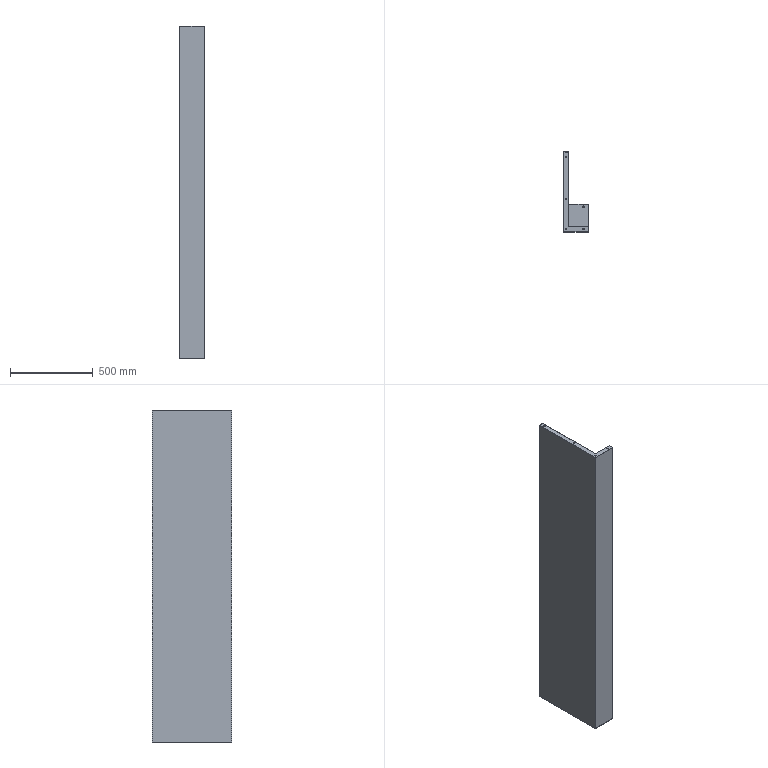Part | SolidWorks | features ICE 8, ExtruThin 1 | 1 solid | 45 faces | box 150 x 480 x 2005 mm | volume 2840339 mm3 | cylinder 30 | plane 15 | commonest cylinder face diameters 9 x30
STEP:
#1=CARTESIAN_POINT('',(148.,16.,1267.5));
#2=VERTEX_POINT('',#1);
#3=CARTESIAN_POINT('',(148.,16.,1258.5));
#4=VERTEX_POINT('',#3);
#5=CARTESIAN_POINT('',(148.,16.,1263.));
#6=DIRECTION('',(1.,0.,0.));
#7=DIRECTION('',(0.,0.,-1.));
#8=AXIS2_PLACEMENT_3D('',#5,#6,#7);
#9=CIRCLE('',#8,4.5);
#10=EDGE_CURVE('',#2,#4,#9,.T.);
#11=ORIENTED_EDGE('',*,*,#10,.F.);
#12=CARTESIAN_POINT('',(150.,16.,1267.5));
#13=VERTEX_POINT('',#12);
#14=CARTESIAN_POINT('',(134.,16.,1267.5));
#15=DIRECTION('',(1.,0.,0.));
#16=VECTOR('',#15,1000.);
#17=LINE('',#14,#16);
#18=EDGE_CURVE('',#2,#13,#17,.T.);
#19=ORIENTED_EDGE('',*,*,#18,.T.);
#20=CARTESIAN_POINT('',(150.,16.,1258.5));
#21=VERTEX_POINT('',#20);
#22=CARTESIAN_POINT('',(150.,16.,1263.));
#23=DIRECTION('',(1.,0.,0.));
#24=DIRECTION('',(0.,0.,-1.));
#25=AXIS2_PLACEMENT_3D('',#22,#23,#24);
#26=CIRCLE('',#25,4.5);
#27=EDGE_CURVE('',#13,#21,#26,.T.);
#28=ORIENTED_EDGE('',*,*,#27,.T.);
#29=CARTESIAN_POINT('',(134.,16.,1258.5));
#30=DIRECTION('',(1.,0.,0.));
#31=VECTOR('',#30,1000.);
#32=LINE('',#29,#31);
#33=EDGE_CURVE('',#4,#21,#32,.T.);
#34=ORIENTED_EDGE('',*,*,#33,.F.);
#35=EDGE_LOOP('',(#11,#19,#28,#34));
#36=FACE_OUTER_BOUND('',#35,.T.);
#37=CARTESIAN_POINT('',(134.,16.,1263.));
#38=DIRECTION('',(1.,0.,0.));
#39=DIRECTION('',(0.,0.,-1.));
#40=AXIS2_PLACEMENT_3D('',#37,#38,#39);
#41=CYLINDRICAL_SURFACE('',#40,4.5);
#42=ADVANCED_FACE('',(#36),#41,.F.);
#43=CARTESIAN_POINT('',(148.,16.,1335.5));
#44=VERTEX_POINT('',#43);
#45=CARTESIAN_POINT('',(148.,16.,1326.5));
#46=VERTEX_POINT('',#45);
#47=CARTESIAN_POINT('',(148.,16.,1331.));
#48=DIRECTION('',(1.,0.,0.));
#49=DIRECTION('',(0.,0.,-1.));
#50=AXIS2_PLACEMENT_3D('',#47,#48,#49);
#51=CIRCLE('',#50,4.5);
#52=EDGE_CURVE('',#44,#46,#51,.T.);
#53=ORIENTED_EDGE('',*,*,#52,.F.);
#54=CARTESIAN_POINT('',(150.,16.,1335.5));
#55=VERTEX_POINT('',#54);
#56=CARTESIAN_POINT('',(134.,16.,1335.5));
#57=DIRECTION('',(1.,0.,0.));
#58=VECTOR('',#57,1000.);
#59=LINE('',#56,#58);
#60=EDGE_CURVE('',#44,#55,#59,.T.);
#61=ORIENTED_EDGE('',*,*,#60,.T.);
#62=CARTESIAN_POINT('',(150.,16.,1326.5));
#63=VERTEX_POINT('',#62);
#64=CARTESIAN_POINT('',(150.,16.,1331.));
#65=DIRECTION('',(1.,0.,0.));
#66=DIRECTION('',(0.,0.,-1.));
#67=AXIS2_PLACEMENT_3D('',#64,#65,#66);
#68=CIRCLE('',#67,4.5);
#69=EDGE_CURVE('',#55,#63,#68,.T.);
#70=ORIENTED_EDGE('',*,*,#69,.T.);
#71=CARTESIAN_POINT('',(134.,16.,1326.5));
#72=DIRECTION('',(1.,0.,0.));
#73=VECTOR('',#72,1000.);
#74=LINE('',#71,#73);
#75=EDGE_CURVE('',#46,#63,#74,.T.);
#76=ORIENTED_EDGE('',*,*,#75,.F.);
#77=EDGE_LOOP('',(#53,#61,#70,#76));
#78=FACE_OUTER_BOUND('',#77,.T.);
#79=CARTESIAN_POINT('',(134.,16.,1331.));
#80=DIRECTION('',(1.,0.,0.));
#81=DIRECTION('',(0.,0.,-1.));
#82=AXIS2_PLACEMENT_3D('',#79,#80,#81);
#83=CYLINDRICAL_SURFACE('',#82,4.5);
#84=ADVANCED_FACE('',(#78),#83,.F.);
#85=CARTESIAN_POINT('',(148.,16.,34.5));
#86=VERTEX_POINT('',#85);
#87=CARTESIAN_POINT('',(148.,16.,25.5));
#88=VERTEX_POINT('',#87);
#89=CARTESIAN_POINT('',(148.,16.,30.));
#90=DIRECTION('',(1.,0.,0.));
#91=DIRECTION('',(0.,0.,-1.));
#92=AXIS2_PLACEMENT_3D('',#89,#90,#91);
#93=CIRCLE('',#92,4.5);
#94=EDGE_CURVE('',#86,#88,#93,.T.);
#95=ORIENTED_EDGE('',*,*,#94,.F.);
#96=CARTESIAN_POINT('',(150.,16.,34.5));
#97=VERTEX_POINT('',#96);
#98=CARTESIAN_POINT('',(134.,16.,34.5));
#99=DIRECTION('',(1.,0.,0.));
#100=VECTOR('',#99,1000.);
#101=LINE('',#98,#100);
#102=EDGE_CURVE('',#86,#97,#101,.T.);
#103=ORIENTED_EDGE('',*,*,#102,.T.);
#104=CARTESIAN_POINT('',(150.,16.,25.5));
#105=VERTEX_POINT('',#104);
#106=CARTESIAN_POINT('',(150.,16.,30.));
#107=DIRECTION('',(1.,0.,0.));
#108=DIRECTION('',(0.,0.,-1.));
#109=AXIS2_PLACEMENT_3D('',#106,#107,#108);
#110=CIRCLE('',#109,4.5);
#111=EDGE_CURVE('',#97,#105,#110,.T.);
#112=ORIENTED_EDGE('',*,*,#111,.T.);
#113=CARTESIAN_POINT('',(134.,16.,25.5));
#114=DIRECTION('',(1.,0.,0.));
#115=VECTOR('',#114,1000.);
#116=LINE('',#113,#115);
#117=EDGE_CURVE('',#88,#105,#116,.T.);
#118=ORIENTED_EDGE('',*,*,#117,.F.);
#119=EDGE_LOOP('',(#95,#103,#112,#118));
#120=FACE_OUTER_BOUND('',#119,.T.);
#121=CARTESIAN_POINT('',(134.,16.,30.));
#122=DIRECTION('',(1.,0.,0.));
#123=DIRECTION('',(0.,0.,-1.));
#124=AXIS2_PLACEMENT_3D('',#121,#122,#123);
#125=CYLINDRICAL_SURFACE('',#124,4.5);
#126=ADVANCED_FACE('',(#120),#125,.F.);
#127=CARTESIAN_POINT('',(148.,16.,179.5));
#128=VERTEX_POINT('',#127);
#129=CARTESIAN_POINT('',(148.,16.,170.5));
#130=VERTEX_POINT('',#129);
#131=CARTESIAN_POINT('',(148.,16.,175.));
#132=DIRECTION('',(1.,0.,0.));
#133=DIRECTION('',(0.,0.,-1.));
#134=AXIS2_PLACEMENT_3D('',#131,#132,#133);
#135=CIRCLE('',#134,4.5);
#136=EDGE_CURVE('',#128,#130,#135,.T.);
#137=ORIENTED_EDGE('',*,*,#136,.F.);
#138=CARTESIAN_POINT('',(150.,16.,179.5));
#139=VERTEX_POINT('',#138);
#140=CARTESIAN_POINT('',(134.,16.,179.5));
#141=DIRECTION('',(1.,0.,0.));
#142=VECTOR('',#141,1000.);
#143=LINE('',#140,#142);
#144=EDGE_CURVE('',#128,#139,#143,.T.);
#145=ORIENTED_EDGE('',*,*,#144,.T.);
#146=CARTESIAN_POINT('',(150.,16.,170.5));
#147=VERTEX_POINT('',#146);
#148=CARTESIAN_POINT('',(150.,16.,175.));
#149=DIRECTION('',(1.,0.,0.));
#150=DIRECTION('',(0.,0.,-1.));
#151=AXIS2_PLACEMENT_3D('',#148,#149,#150);
#152=CIRCLE('',#151,4.5);
#153=EDGE_CURVE('',#139,#147,#152,.T.);
#154=ORIENTED_EDGE('',*,*,#153,.T.);
#155=CARTESIAN_POINT('',(134.,16.,170.5));
#156=DIRECTION('',(1.,0.,0.));
#157=VECTOR('',#156,1000.);
#158=LINE('',#155,#157);
#159=EDGE_CURVE('',#130,#147,#158,.T.);
#160=ORIENTED_EDGE('',*,*,#159,.F.);
#161=EDGE_LOOP('',(#137,#145,#154,#160));
#162=FACE_OUTER_BOUND('',#161,.T.);
#163=CARTESIAN_POINT('',(134.,16.,175.));
#164=DIRECTION('',(1.,0.,0.));
#165=DIRECTION('',(0.,0.,-1.));
#166=AXIS2_PLACEMENT_3D('',#163,#164,#165);
#167=CYLINDRICAL_SURFACE('',#166,4.5);
#168=ADVANCED_FACE('',(#162),#167,.F.);
#169=CARTESIAN_POINT('',(115.5,16.,2003.));
#170=VERTEX_POINT('',#169);
#171=CARTESIAN_POINT('',(124.5,16.,2003.));
#172=VERTEX_POINT('',#171);
#173=CARTESIAN_POINT('',(120.,16.,2003.));
#174=DIRECTION('',(0.,0.,1.));
#175=DIRECTION('',(1.,0.,0.));
#176=AXIS2_PLACEMENT_3D('',#173,#174,#175);
#177=CIRCLE('',#176,4.5);
#178=EDGE_CURVE('',#170,#172,#177,.T.);
#179=ORIENTED_EDGE('',*,*,#178,.F.);
#180=CARTESIAN_POINT('',(115.5,16.,2005.));
#181=VERTEX_POINT('',#180);
#182=CARTESIAN_POINT('',(115.5,16.,1995.));
#183=DIRECTION('',(0.,0.,1.));
#184=VECTOR('',#183,1000.);
#185=LINE('',#182,#184);
#186=EDGE_CURVE('',#170,#181,#185,.T.);
#187=ORIENTED_EDGE('',*,*,#186,.T.);
#188=CARTESIAN_POINT('',(124.5,16.,2005.));
#189=VERTEX_POINT('',#188);
#190=CARTESIAN_POINT('',(120.,16.,2005.));
#191=DIRECTION('',(0.,0.,1.));
#192=DIRECTION('',(1.,0.,0.));
#193=AXIS2_PLACEMENT_3D('',#190,#191,#192);
#194=CIRCLE('',#193,4.5);
#195=EDGE_CURVE('',#181,#189,#194,.T.);
#196=ORIENTED_EDGE('',*,*,#195,.T.);
#197=CARTESIAN_POINT('',(124.5,16.,1995.));
#198=DIRECTION('',(0.,0.,1.));
#199=VECTOR('',#198,1000.);
#200=LINE('',#197,#199);
#201=EDGE_CURVE('',#172,#189,#200,.T.);
#202=ORIENTED_EDGE('',*,*,#201,.F.);
#203=EDGE_LOOP('',(#179,#187,#196,#202));
#204=FACE_OUTER_BOUND('',#203,.T.);
#205=CARTESIAN_POINT('',(120.,16.,1995.));
#206=DIRECTION('',(0.,0.,1.));
#207=DIRECTION('',(1.,0.,0.));
#208=AXIS2_PLACEMENT_3D('',#205,#206,#207);
#209=CYLINDRICAL_SURFACE('',#208,4.5);
#210=ADVANCED_FACE('',(#204),#209,.F.);
#211=CARTESIAN_POINT('',(11.5,16.,2003.));
#212=VERTEX_POINT('',#211);
#213=CARTESIAN_POINT('',(20.5,16.,2003.));
#214=VERTEX_POINT('',#213);
#215=CARTESIAN_POINT('',(16.,16.,2003.));
#216=DIRECTION('',(0.,0.,1.));
#217=DIRECTION('',(1.,0.,0.));
#218=AXIS2_PLACEMENT_3D('',#215,#216,#217);
#219=CIRCLE('',#218,4.5);
#220=EDGE_CURVE('',#212,#214,#219,.T.);
#221=ORIENTED_EDGE('',*,*,#220,.F.);
#222=CARTESIAN_POINT('',(11.5,16.,2005.));
#223=VERTEX_POINT('',#222);
#224=CARTESIAN_POINT('',(11.5,16.,1995.));
#225=DIRECTION('',(0.,0.,1.));
#226=VECTOR('',#225,1000.);
#227=LINE('',#224,#226);
#228=EDGE_CURVE('',#212,#223,#227,.T.);
#229=ORIENTED_EDGE('',*,*,#228,.T.);
#230=CARTESIAN_POINT('',(20.5,16.,2005.));
#231=VERTEX_POINT('',#230);
#232=CARTESIAN_POINT('',(16.,16.,2005.));
#233=DIRECTION('',(0.,0.,1.));
#234=DIRECTION('',(1.,0.,0.));
#235=AXIS2_PLACEMENT_3D('',#232,#233,#234);
#236=CIRCLE('',#235,4.5);
#237=EDGE_CURVE('',#223,#231,#236,.T.);
#238=ORIENTED_EDGE('',*,*,#237,.T.);
#239=CARTESIAN_POINT('',(20.5,16.,1995.));
#240=DIRECTION('',(0.,0.,1.));
#241=VECTOR('',#240,1000.);
#242=LINE('',#239,#241);
#243=EDGE_CURVE('',#214,#231,#242,.T.);
#244=ORIENTED_EDGE('',*,*,#243,.F.);
#245=EDGE_LOOP('',(#221,#229,#238,#244));
#246=FACE_OUTER_BOUND('',#245,.T.);
#247=CARTESIAN_POINT('',(16.,16.,1995.));
#248=DIRECTION('',(0.,0.,1.));
#249=DIRECTION('',(1.,0.,0.));
#250=AXIS2_PLACEMENT_3D('',#247,#248,#249);
#251=CYLINDRICAL_SURFACE('',#250,4.5);
#252=ADVANCED_FACE('',(#246),#251,.F.);
#253=CARTESIAN_POINT('',(11.5,197.,2003.));
#254=VERTEX_POINT('',#253);
#255=CARTESIAN_POINT('',(20.5,197.,2003.));
#256=VERTEX_POINT('',#255);
#257=CARTESIAN_POINT('',(16.,197.,2003.));
#258=DIRECTION('',(0.,0.,1.));
#259=DIRECTION('',(1.,0.,0.));
#260=AXIS2_PLACEMENT_3D('',#257,#258,#259);
#261=CIRCLE('',#260,4.5);
#262=EDGE_CURVE('',#254,#256,#261,.T.);
#263=ORIENTED_EDGE('',*,*,#262,.F.);
#264=CARTESIAN_POINT('',(11.5,197.,2005.));
#265=VERTEX_POINT('',#264);
#266=CARTESIAN_POINT('',(11.5,197.,1995.));
#267=DIRECTION('',(0.,0.,1.));
#268=VECTOR('',#267,1000.);
#269=LINE('',#266,#268);
#270=EDGE_CURVE('',#254,#265,#269,.T.);
#271=ORIENTED_EDGE('',*,*,#270,.T.);
#272=CARTESIAN_POINT('',(20.5,197.,2005.));
#273=VERTEX_POINT('',#272);
#274=CARTESIAN_POINT('',(16.,197.,2005.));
#275=DIRECTION('',(0.,0.,1.));
#276=DIRECTION('',(1.,0.,0.));
#277=AXIS2_PLACEMENT_3D('',#274,#275,#276);
#278=CIRCLE('',#277,4.5);
#279=EDGE_CURVE('',#265,#273,#278,.T.);
#280=ORIENTED_EDGE('',*,*,#279,.T.);
#281=CARTESIAN_POINT('',(20.5,197.,1995.));
#282=DIRECTION('',(0.,0.,1.));
#283=VECTOR('',#282,1000.);
#284=LINE('',#281,#283);
#285=EDGE_CURVE('',#256,#273,#284,.T.);
#286=ORIENTED_EDGE('',*,*,#285,.F.);
#287=EDGE_LOOP('',(#263,#271,#280,#286));
#288=FACE_OUTER_BOUND('',#287,.T.);
#289=CARTESIAN_POINT('',(16.,197.,1995.));
#290=DIRECTION('',(0.,0.,1.));
#291=DIRECTION('',(1.,0.,0.));
#292=AXIS2_PLACEMENT_3D('',#289,#290,#291);
#293=CYLINDRICAL_SURFACE('',#292,4.5);
#294=ADVANCED_FACE('',(#288),#293,.F.);
#295=CARTESIAN_POINT('',(11.5,450.,2003.));
#296=VERTEX_POINT('',#295);
#297=CARTESIAN_POINT('',(20.5,450.,2003.));
#298=VERTEX_POINT('',#297);
#299=CARTESIAN_POINT('',(16.,450.,2003.));
#300=DIRECTION('',(0.,0.,1.));
#301=DIRECTION('',(1.,0.,0.));
#302=AXIS2_PLACEMENT_3D('',#299,#300,#301);
#303=CIRCLE('',#302,4.5);
#304=EDGE_CURVE('',#296,#298,#303,.T.);
#305=ORIENTED_EDGE('',*,*,#304,.F.);
#306=CARTESIAN_POINT('',(11.5,450.,2005.));
#307=VERTEX_POINT('',#306);
#308=CARTESIAN_POINT('',(11.5,450.,1995.));
#309=DIRECTION('',(0.,0.,1.));
#310=VECTOR('',#309,1000.);
#311=LINE('',#308,#310);
#312=EDGE_CURVE('',#296,#307,#311,.T.);
#313=ORIENTED_EDGE('',*,*,#312,.T.);
#314=CARTESIAN_POINT('',(20.5,450.,2005.));
#315=VERTEX_POINT('',#314);
#316=CARTESIAN_POINT('',(16.,450.,2005.));
#317=DIRECTION('',(0.,0.,1.));
#318=DIRECTION('',(1.,0.,0.));
#319=AXIS2_PLACEMENT_3D('',#316,#317,#318);
#320=CIRCLE('',#319,4.5);
#321=EDGE_CURVE('',#307,#315,#320,.T.);
#322=ORIENTED_EDGE('',*,*,#321,.T.);
#323=CARTESIAN_POINT('',(20.5,450.,1995.));
#324=DIRECTION('',(0.,0.,1.));
#325=VECTOR('',#324,1000.);
#326=LINE('',#323,#325);
#327=EDGE_CURVE('',#298,#315,#326,.T.);
#328=ORIENTED_EDGE('',*,*,#327,.F.);
#329=EDGE_LOOP('',(#305,#313,#322,#328));
#330=FACE_OUTER_BOUND('',#329,.T.);
#331=CARTESIAN_POINT('',(16.,450.,1995.));
#332=DIRECTION('',(0.,0.,1.));
#333=DIRECTION('',(1.,0.,0.));
#334=AXIS2_PLACEMENT_3D('',#331,#332,#333);
#335=CYLINDRICAL_SURFACE('',#334,4.5);
#336=ADVANCED_FACE('',(#330),#335,.F.);
#337=CARTESIAN_POINT('',(20.5,480.,1563.));
#338=VERTEX_POINT('',#337);
#339=CARTESIAN_POINT('',(11.5,480.,1563.));
#340=VERTEX_POINT('',#339);
#341=CARTESIAN_POINT('',(16.,480.,1563.));
#342=DIRECTION('',(0.,1.,0.));
#343=DIRECTION('',(0.,0.,1.));
#344=AXIS2_PLACEMENT_3D('',#341,#342,#343);
#345=CIRCLE('',#344,4.5);
#346=EDGE_CURVE('',#338,#340,#345,.T.);
#347=ORIENTED_EDGE('',*,*,#346,.T.);
#348=CARTESIAN_POINT('',(11.5,478.,1563.));
#349=VERTEX_POINT('',#348);
#350=CARTESIAN_POINT('',(11.5,488.,1563.));
#351=DIRECTION('',(0.,-1.,0.));
#352=VECTOR('',#351,1000.);
#353=LINE('',#350,#352);
#354=EDGE_CURVE('',#340,#349,#353,.T.);
#355=ORIENTED_EDGE('',*,*,#354,.T.);
#356=CARTESIAN_POINT('',(20.5,478.,1563.));
#357=VERTEX_POINT('',#356);
#358=CARTESIAN_POINT('',(16.,478.,1563.));
#359=DIRECTION('',(0.,-1.,0.));
#360=DIRECTION('',(1.,0.,0.));
#361=AXIS2_PLACEMENT_3D('',#358,#359,#360);
#362=CIRCLE('',#361,4.5);
#363=EDGE_CURVE('',#349,#357,#362,.T.);
#364=ORIENTED_EDGE('',*,*,#363,.T.);
#365=CARTESIAN_POINT('',(20.5,488.,1563.));
#366=DIRECTION('',(0.,-1.,0.));
#367=VECTOR('',#366,1000.);
#368=LINE('',#365,#367);
#369=EDGE_CURVE('',#338,#357,#368,.T.);
#370=ORIENTED_EDGE('',*,*,#369,.F.);
#371=EDGE_LOOP('',(#347,#355,#364,#370));
#372=FACE_OUTER_BOUND('',#371,.T.);
#373=CARTESIAN_POINT('',(16.,488.,1563.));
#374=DIRECTION('',(0.,-1.,0.));
#375=DIRECTION('',(1.,0.,0.));
#376=AXIS2_PLACEMENT_3D('',#373,#374,#375);
#377=CYLINDRICAL_SURFACE('',#376,4.5);
#378=ADVANCED_FACE('',(#372),#377,.F.);
#379=CARTESIAN_POINT('',(20.5,480.,1975.));
#380=VERTEX_POINT('',#379);
#381=CARTESIAN_POINT('',(11.5,480.,1975.));
#382=VERTEX_POINT('',#381);
#383=CARTESIAN_POINT('',(16.,480.,1975.));
#384=DIRECTION('',(0.,1.,0.));
#385=DIRECTION('',(0.,0.,1.));
#386=AXIS2_PLACEMENT_3D('',#383,#384,#385);
#387=CIRCLE('',#386,4.5);
#388=EDGE_CURVE('',#380,#382,#387,.T.);
#389=ORIENTED_EDGE('',*,*,#388,.T.);
#390=CARTESIAN_POINT('',(11.5,478.,1975.));
#391=VERTEX_POINT('',#390);
#392=CARTESIAN_POINT('',(11.5,488.,1975.));
#393=DIRECTION('',(0.,-1.,0.));
#394=VECTOR('',#393,1000.);
#395=LINE('',#392,#394);
#396=EDGE_CURVE('',#382,#391,#395,.T.);
#397=ORIENTED_EDGE('',*,*,#396,.T.);
#398=CARTESIAN_POINT('',(20.5,478.,1975.));
#399=VERTEX_POINT('',#398);
#400=CARTESIAN_POINT('',(16.,478.,1975.));
#401=DIRECTION('',(0.,-1.,0.));
#402=DIRECTION('',(1.,0.,0.));
#403=AXIS2_PLACEMENT_3D('',#400,#401,#402);
#404=CIRCLE('',#403,4.5);
#405=EDGE_CURVE('',#391,#399,#404,.T.);
#406=ORIENTED_EDGE('',*,*,#405,.T.);
#407=CARTESIAN_POINT('',(20.5,488.,1975.));
#408=DIRECTION('',(0.,-1.,0.));
#409=VECTOR('',#408,1000.);
#410=LINE('',#407,#409);
#411=EDGE_CURVE('',#380,#399,#410,.T.);
#412=ORIENTED_EDGE('',*,*,#411,.F.);
#413=EDGE_LOOP('',(#389,#397,#406,#412));
#414=FACE_OUTER_BOUND('',#413,.T.);
#415=CARTESIAN_POINT('',(16.,488.,1975.));
#416=DIRECTION('',(0.,-1.,0.));
#417=DIRECTION('',(1.,0.,0.));
#418=AXIS2_PLACEMENT_3D('',#415,#416,#417);
#419=CYLINDRICAL_SURFACE('',#418,4.5);
#420=ADVANCED_FACE('',(#414),#419,.F.);
#421=CARTESIAN_POINT('',(20.5,480.,180.));
#422=VERTEX_POINT('',#421);
#423=CARTESIAN_POINT('',(11.5,480.,180.));
#424=VERTEX_POINT('',#423);
#425=CARTESIAN_POINT('',(16.,480.,180.));
#426=DIRECTION('',(0.,1.,0.));
#427=DIRECTION('',(0.,0.,1.));
#428=AXIS2_PLACEMENT_3D('',#425,#426,#427);
#429=CIRCLE('',#428,4.5);
#430=EDGE_CURVE('',#422,#424,#429,.T.);
#431=ORIENTED_EDGE('',*,*,#430,.T.);
#432=CARTESIAN_POINT('',(11.5,478.,180.));
#433=VERTEX_POINT('',#432);
#434=CARTESIAN_POINT('',(11.5,554.,180.));
#435=DIRECTION('',(0.,-1.,0.));
#436=VECTOR('',#435,1000.);
#437=LINE('',#434,#436);
#438=EDGE_CURVE('',#424,#433,#437,.T.);
#439=ORIENTED_EDGE('',*,*,#438,.T.);
#440=CARTESIAN_POINT('',(20.5,478.,180.));
#441=VERTEX_POINT('',#440);
#442=CARTESIAN_POINT('',(16.,478.,180.));
#443=DIRECTION('',(0.,-1.,0.));
#444=DIRECTION('',(1.,0.,0.));
#445=AXIS2_PLACEMENT_3D('',#442,#443,#444);
#446=CIRCLE('',#445,4.5);
#447=EDGE_CURVE('',#433,#441,#446,.T.);
#448=ORIENTED_EDGE('',*,*,#447,.T.);
#449=CARTESIAN_POINT('',(20.5,554.,180.));
#450=DIRECTION('',(0.,-1.,0.));
#451=VECTOR('',#450,1000.);
#452=LINE('',#449,#451);
#453=EDGE_CURVE('',#422,#441,#452,.T.);
#454=ORIENTED_EDGE('',*,*,#453,.F.);
#455=EDGE_LOOP('',(#431,#439,#448,#454));
#456=FACE_OUTER_BOUND('',#455,.T.);
#457=CARTESIAN_POINT('',(16.,554.,180.));
#458=DIRECTION('',(0.,-1.,0.));
#459=DIRECTION('',(1.,0.,0.));
#460=AXIS2_PLACEMENT_3D('',#457,#458,#459);
#461=CYLINDRICAL_SURFACE('',#460,4.5);
#462=ADVANCED_FACE('',(#456),#461,.F.);
#463=CARTESIAN_POINT('',(20.5,480.,30.));
#464=VERTEX_POINT('',#463);
#465=CARTESIAN_POINT('',(11.5,480.,30.));
#466=VERTEX_POINT('',#465);
#467=CARTESIAN_POINT('',(16.,480.,30.));
#468=DIRECTION('',(0.,1.,0.));
#469=DIRECTION('',(0.,0.,1.));
#470=AXIS2_PLACEMENT_3D('',#467,#468,#469);
#471=CIRCLE('',#470,4.5);
#472=EDGE_CURVE('',#464,#466,#471,.T.);
#473=ORIENTED_EDGE('',*,*,#472,.T.);
#474=CARTESIAN_POINT('',(11.5,478.,30.));
#475=VERTEX_POINT('',#474);
#476=CARTESIAN_POINT('',(11.5,554.,30.));
#477=DIRECTION('',(0.,-1.,0.));
#478=VECTOR('',#477,1000.);
#479=LINE('',#476,#478);
#480=EDGE_CURVE('',#466,#475,#479,.T.);
#481=ORIENTED_EDGE('',*,*,#480,.T.);
#482=CARTESIAN_POINT('',(20.5,478.,30.));
#483=VERTEX_POINT('',#482);
#484=CARTESIAN_POINT('',(16.,478.,30.));
#485=DIRECTION('',(0.,-1.,0.));
#486=DIRECTION('',(1.,0.,0.));
#487=AXIS2_PLACEMENT_3D('',#484,#485,#486);
#488=CIRCLE('',#487,4.5);
#489=EDGE_CURVE('',#475,#483,#488,.T.);
#490=ORIENTED_EDGE('',*,*,#489,.T.);
#491=CARTESIAN_POINT('',(20.5,554.,30.));
#492=DIRECTION('',(0.,-1.,0.));
#493=VECTOR('',#492,1000.);
#494=LINE('',#491,#493);
#495=EDGE_CURVE('',#464,#483,#494,.T.);
#496=ORIENTED_EDGE('',*,*,#495,.F.);
#497=EDGE_LOOP('',(#473,#481,#490,#496));
#498=FACE_OUTER_BOUND('',#497,.T.);
#499=CARTESIAN_POINT('',(16.,554.,30.));
#500=DIRECTION('',(0.,-1.,0.));
#501=DIRECTION('',(1.,0.,0.));
#502=AXIS2_PLACEMENT_3D('',#499,#500,#501);
#503=CYLINDRICAL_SURFACE('',#502,4.5);
#504=ADVANCED_FACE('',(#498),#503,.F.);
#505=CARTESIAN_POINT('',(20.5,250.,0.));
#506=VERTEX_POINT('',#505);
#507=CARTESIAN_POINT('',(11.5,250.,0.));
#508=VERTEX_POINT('',#507);
#509=CARTESIAN_POINT('',(16.,250.,0.));
#510=DIRECTION('',(0.,0.,-1.));
#511=DIRECTION('',(-1.,0.,0.));
#512=AXIS2_PLACEMENT_3D('',#509,#510,#511);
#513=CIRCLE('',#512,4.5);
#514=EDGE_CURVE('',#506,#508,#513,.T.);
#515=ORIENTED_EDGE('',*,*,#514,.T.);
#516=CARTESIAN_POINT('',(11.5,250.,2.));
#517=VERTEX_POINT('',#516);
#518=CARTESIAN_POINT('',(11.5,250.,-8.));
#519=DIRECTION('',(0.,0.,1.));
#520=VECTOR('',#519,1000.);
#521=LINE('',#518,#520);
#522=EDGE_CURVE('',#508,#517,#521,.T.);
#523=ORIENTED_EDGE('',*,*,#522,.T.);
#524=CARTESIAN_POINT('',(20.5,250.,2.));
#525=VERTEX_POINT('',#524);
#526=CARTESIAN_POINT('',(16.,250.,2.));
#527=DIRECTION('',(0.,0.,1.));
#528=DIRECTION('',(1.,0.,0.));
#529=AXIS2_PLACEMENT_3D('',#526,#527,#528);
#530=CIRCLE('',#529,4.5);
#531=EDGE_CURVE('',#517,#525,#530,.T.);
#532=ORIENTED_EDGE('',*,*,#531,.T.);
#533=CARTESIAN_POINT('',(20.5,250.,-8.));
#534=DIRECTION('',(0.,0.,1.));
#535=VECTOR('',#534,1000.);
#536=LINE('',#533,#535);
#537=EDGE_CURVE('',#506,#525,#536,.T.);
#538=ORIENTED_EDGE('',*,*,#537,.F.);
#539=EDGE_LOOP('',(#515,#523,#532,#538));
#540=FACE_OUTER_BOUND('',#539,.T.);
#541=CARTESIAN_POINT('',(16.,250.,-8.));
#542=DIRECTION('',(0.,0.,1.));
#543=DIRECTION('',(1.,0.,0.));
#544=AXIS2_PLACEMENT_3D('',#541,#542,#543);
#545=CYLINDRICAL_SURFACE('',#544,4.5);
#546=ADVANCED_FACE('',(#540),#545,.F.);
#547=CARTESIAN_POINT('',(20.5,450.,0.));
#548=VERTEX_POINT('',#547);
#549=CARTESIAN_POINT('',(11.5,450.,0.));
#550=VERTEX_POINT('',#549);
#551=CARTESIAN_POINT('',(16.,450.,0.));
#552=DIRECTION('',(0.,0.,-1.));
#553=DIRECTION('',(-1.,0.,0.));
#554=AXIS2_PLACEMENT_3D('',#551,#552,#553);
#555=CIRCLE('',#554,4.5);
#556=EDGE_CURVE('',#548,#550,#555,.T.);
#557=ORIENTED_EDGE('',*,*,#556,.T.);
#558=CARTESIAN_POINT('',(11.5,450.,2.));
#559=VERTEX_POINT('',#558);
#560=CARTESIAN_POINT('',(11.5,450.,-8.));
#561=DIRECTION('',(0.,0.,1.));
#562=VECTOR('',#561,1000.);
#563=LINE('',#560,#562);
#564=EDGE_CURVE('',#550,#559,#563,.T.);
#565=ORIENTED_EDGE('',*,*,#564,.T.);
#566=CARTESIAN_POINT('',(20.5,450.,2.));
#567=VERTEX_POINT('',#566);
#568=CARTESIAN_POINT('',(16.,450.,2.));
#569=DIRECTION('',(0.,0.,1.));
#570=DIRECTION('',(1.,0.,0.));
#571=AXIS2_PLACEMENT_3D('',#568,#569,#570);
#572=CIRCLE('',#571,4.5);
#573=EDGE_CURVE('',#559,#567,#572,.T.);
#574=ORIENTED_EDGE('',*,*,#573,.T.);
#575=CARTESIAN_POINT('',(20.5,450.,-8.));
#576=DIRECTION('',(0.,0.,1.));
#577=VECTOR('',#576,1000.);
#578=LINE('',#575,#577);
#579=EDGE_CURVE('',#548,#567,#578,.T.);
#580=ORIENTED_EDGE('',*,*,#579,.F.);
#581=EDGE_LOOP('',(#557,#565,#574,#580));
#582=FACE_OUTER_BOUND('',#581,.T.);
#583=CARTESIAN_POINT('',(16.,450.,-8.));
#584=DIRECTION('',(0.,0.,1.));
#585=DIRECTION('',(1.,0.,0.));
#586=AXIS2_PLACEMENT_3D('',#583,#584,#585);
#587=CYLINDRICAL_SURFACE('',#586,4.5);
#588=ADVANCED_FACE('',(#582),#587,.F.);
#589=CARTESIAN_POINT('',(124.5,153.,0.));
#590=VERTEX_POINT('',#589);
#591=CARTESIAN_POINT('',(115.5,153.,0.));
#592=VERTEX_POINT('',#591);
#593=CARTESIAN_POINT('',(120.,153.,0.));
#594=DIRECTION('',(0.,0.,-1.));
#595=DIRECTION('',(-1.,0.,0.));
#596=AXIS2_PLACEMENT_3D('',#593,#594,#595);
#597=CIRCLE('',#596,4.5);
#598=EDGE_CURVE('',#590,#592,#597,.T.);
#599=ORIENTED_EDGE('',*,*,#598,.T.);
#600=CARTESIAN_POINT('',(115.5,153.,2.));
#601=VERTEX_POINT('',#600);
#602=CARTESIAN_POINT('',(115.5,153.,-8.));
#603=DIRECTION('',(0.,0.,1.));
#604=VECTOR('',#603,1000.);
#605=LINE('',#602,#604);
#606=EDGE_CURVE('',#592,#601,#605,.T.);
#607=ORIENTED_EDGE('',*,*,#606,.T.);
#608=CARTESIAN_POINT('',(124.5,153.,2.));
#609=VERTEX_POINT('',#608);
#610=CARTESIAN_POINT('',(120.,153.,2.));
#611=DIRECTION('',(0.,0.,1.));
#612=DIRECTION('',(1.,0.,0.));
#613=AXIS2_PLACEMENT_3D('',#610,#611,#612);
#614=CIRCLE('',#613,4.5);
#615=EDGE_CURVE('',#601,#609,#614,.T.);
#616=ORIENTED_EDGE('',*,*,#615,.T.);
#617=CARTESIAN_POINT('',(124.5,153.,-8.));
#618=DIRECTION('',(0.,0.,1.));
#619=VECTOR('',#618,1000.);
#620=LINE('',#617,#619);
#621=EDGE_CURVE('',#590,#609,#620,.T.);
#622=ORIENTED_EDGE('',*,*,#621,.F.);
#623=EDGE_LOOP('',(#599,#607,#616,#622));
#624=FACE_OUTER_BOUND('',#623,.T.);
#625=CARTESIAN_POINT('',(120.,153.,-8.));
#626=DIRECTION('',(0.,0.,1.));
#627=DIRECTION('',(1.,0.,0.));
#628=AXIS2_PLACEMENT_3D('',#625,#626,#627);
#629=CYLINDRICAL_SURFACE('',#628,4.5);
#630=ADVANCED_FACE('',(#624),#629,.F.);
#631=CARTESIAN_POINT('',(148.,2.,2.));
#632=VERTEX_POINT('',#631);
#633=CARTESIAN_POINT('',(148.,2.,2003.));
#634=VERTEX_POINT('',#633);
#635=CARTESIAN_POINT('',(148.,2.,2003.));
#636=DIRECTION('',(0.,0.,1.));
#637=VECTOR('',#636,1000.);
#638=LINE('',#635,#637);
#639=EDGE_CURVE('',#632,#634,#638,.T.);
#640=ORIENTED_EDGE('',*,*,#639,.F.);
#641=CARTESIAN_POINT('',(2.,2.,2.));
#642=VERTEX_POINT('',#641);
#643=CARTESIAN_POINT('',(30.,2.,2.));
#644=DIRECTION('',(-1.,0.,0.));
#645=VECTOR('',#644,1000.);
#646=LINE('',#643,#645);
#647=EDGE_CURVE('',#632,#642,#646,.T.);
#648=ORIENTED_EDGE('',*,*,#647,.T.);
#649=CARTESIAN_POINT('',(2.,2.,2003.));
#650=VERTEX_POINT('',#649);
#651=CARTESIAN_POINT('',(2.,2.,2005.));
#652=DIRECTION('',(0.,0.,-1.));
#653=VECTOR('',#652,1000.);
#654=LINE('',#651,#653);
#655=EDGE_CURVE('',#650,#642,#654,.T.);
#656=ORIENTED_EDGE('',*,*,#655,.F.);
#657=CARTESIAN_POINT('',(30.,2.,2003.));
#658=DIRECTION('',(-1.,0.,0.));
#659=VECTOR('',#658,1000.);
#660=LINE('',#657,#659);
#661=EDGE_CURVE('',#634,#650,#660,.T.);
#662=ORIENTED_EDGE('',*,*,#661,.F.);
#663=EDGE_LOOP('',(#640,#648,#656,#662));
#664=FACE_OUTER_BOUND('',#663,.T.);
#665=CARTESIAN_POINT('',(0.,2.,2005.));
#666=DIRECTION('',(0.,1.,0.));
#667=DIRECTION('',(0.,0.,1.));
#668=AXIS2_PLACEMENT_3D('',#665,#666,#667);
#669=PLANE('',#668);
#670=ADVANCED_FACE('',(#664),#669,.T.);
#671=CARTESIAN_POINT('',(30.,167.,0.));
#672=VERTEX_POINT('',#671);
#673=CARTESIAN_POINT('',(30.,167.,2.));
#674=VERTEX_POINT('',#673);
#675=CARTESIAN_POINT('',(30.,167.,0.));
#676=DIRECTION('',(0.,0.,1.));
#677=VECTOR('',#676,1000.);
#678=LINE('',#675,#677);
#679=EDGE_CURVE('',#672,#674,#678,.T.);
#680=ORIENTED_EDGE('',*,*,#679,.F.);
#681=CARTESIAN_POINT('',(30.,480.,0.));
#682=VERTEX_POINT('',#681);
#683=CARTESIAN_POINT('',(30.,480.,0.));
#684=DIRECTION('',(0.,1.,0.));
#685=VECTOR('',#684,1000.);
#686=LINE('',#683,#685);
#687=EDGE_CURVE('',#672,#682,#686,.T.);
#688=ORIENTED_EDGE('',*,*,#687,.T.);
#689=CARTESIAN_POINT('',(30.,480.,2005.));
#690=VERTEX_POINT('',#689);
#691=CARTESIAN_POINT('',(30.,480.,2005.));
#692=DIRECTION('',(0.,0.,1.));
#693=VECTOR('',#692,1000.);
#694=LINE('',#691,#693);
#695=EDGE_CURVE('',#682,#690,#694,.T.);
#696=ORIENTED_EDGE('',*,*,#695,.T.);
#697=CARTESIAN_POINT('',(30.,30.,2005.));
#698=VERTEX_POINT('',#697);
#699=CARTESIAN_POINT('',(30.,2.,2005.));
#700=DIRECTION('',(0.,-1.,0.));
#701=VECTOR('',#700,1000.);
#702=LINE('',#699,#701);
#703=EDGE_CURVE('',#690,#698,#702,.T.);
#704=ORIENTED_EDGE('',*,*,#703,.T.);
#705=CARTESIAN_POINT('',(30.,30.,2003.));
#706=VERTEX_POINT('',#705);
#707=CARTESIAN_POINT('',(30.,30.,2003.));
#708=DIRECTION('',(0.,0.,1.));
#709=VECTOR('',#708,1000.);
#710=LINE('',#707,#709);
#711=EDGE_CURVE('',#706,#698,#710,.T.);
#712=ORIENTED_EDGE('',*,*,#711,.F.);
#713=CARTESIAN_POINT('',(30.,478.,2003.));
#714=VERTEX_POINT('',#713);
#715=CARTESIAN_POINT('',(30.,2.,2003.));
#716=DIRECTION('',(0.,1.,0.));
#717=VECTOR('',#716,1000.);
#718=LINE('',#715,#717);
#719=EDGE_CURVE('',#706,#714,#718,.T.);
#720=ORIENTED_EDGE('',*,*,#719,.T.);
#721=CARTESIAN_POINT('',(30.,478.,2.));
#722=VERTEX_POINT('',#721);
#723=CARTESIAN_POINT('',(30.,478.,2003.));
#724=DIRECTION('',(0.,0.,-1.));
#725=VECTOR('',#724,1000.);
#726=LINE('',#723,#725);
#727=EDGE_CURVE('',#714,#722,#726,.T.);
#728=ORIENTED_EDGE('',*,*,#727,.T.);
#729=CARTESIAN_POINT('',(30.,478.,2.));
#730=DIRECTION('',(0.,-1.,0.));
#731=VECTOR('',#730,1000.);
#732=LINE('',#729,#731);
#733=EDGE_CURVE('',#722,#674,#732,.T.);
#734=ORIENTED_EDGE('',*,*,#733,.T.);
#735=EDGE_LOOP('',(#680,#688,#696,#704,#712,#720,#728,#734));
#736=FACE_OUTER_BOUND('',#735,.T.);
#737=CARTESIAN_POINT('',(30.,480.,2005.));
#738=DIRECTION('',(-1.,0.,0.));
#739=DIRECTION('',(0.,-1.,0.));
#740=AXIS2_PLACEMENT_3D('',#737,#738,#739);
#741=PLANE('',#740);
#742=ADVANCED_FACE('',(#736),#741,.F.);
#743=CARTESIAN_POINT('',(148.,16.,1263.));
#744=DIRECTION('',(1.,0.,0.));
#745=DIRECTION('',(0.,0.,-1.));
#746=AXIS2_PLACEMENT_3D('',#743,#744,#745);
#747=CIRCLE('',#746,4.5);
#748=EDGE_CURVE('',#4,#2,#747,.T.);
#749=ORIENTED_EDGE('',*,*,#748,.T.);
#750=ORIENTED_EDGE('',*,*,#10,.T.);
#751=EDGE_LOOP('',(#749,#750));
#752=FACE_BOUND('',#751,.T.);
#753=CARTESIAN_POINT('',(148.,16.,1331.));
#754=DIRECTION('',(1.,0.,0.));
#755=DIRECTION('',(0.,0.,-1.));
#756=AXIS2_PLACEMENT_3D('',#753,#754,#755);
#757=CIRCLE('',#756,4.5);
#758=EDGE_CURVE('',#46,#44,#757,.T.);
#759=ORIENTED_EDGE('',*,*,#758,.T.);
#760=ORIENTED_EDGE('',*,*,#52,.T.);
#761=EDGE_LOOP('',(#759,#760));
#762=FACE_BOUND('',#761,.T.);
#763=CARTESIAN_POINT('',(148.,16.,30.));
#764=DIRECTION('',(1.,0.,0.));
#765=DIRECTION('',(0.,0.,-1.));
#766=AXIS2_PLACEMENT_3D('',#763,#764,#765);
#767=CIRCLE('',#766,4.5);
#768=EDGE_CURVE('',#88,#86,#767,.T.);
#769=ORIENTED_EDGE('',*,*,#768,.T.);
#770=ORIENTED_EDGE('',*,*,#94,.T.);
#771=EDGE_LOOP('',(#769,#770));
#772=FACE_BOUND('',#771,.T.);
#773=CARTESIAN_POINT('',(148.,16.,175.));
#774=DIRECTION('',(1.,0.,0.));
#775=DIRECTION('',(0.,0.,-1.));
#776=AXIS2_PLACEMENT_3D('',#773,#774,#775);
#777=CIRCLE('',#776,4.5);
#778=EDGE_CURVE('',#130,#128,#777,.T.);
#779=ORIENTED_EDGE('',*,*,#778,.T.);
#780=ORIENTED_EDGE('',*,*,#136,.T.);
#781=EDGE_LOOP('',(#779,#780));
#782=FACE_BOUND('',#781,.T.);
#783=CARTESIAN_POINT('',(148.,30.,2.));
#784=VERTEX_POINT('',#783);
#785=CARTESIAN_POINT('',(148.,30.,2.));
#786=DIRECTION('',(0.,1.,0.));
#787=VECTOR('',#786,1000.);
#788=LINE('',#785,#787);
#789=EDGE_CURVE('',#632,#784,#788,.T.);
#790=ORIENTED_EDGE('',*,*,#789,.F.);
#791=ORIENTED_EDGE('',*,*,#639,.T.);
#792=CARTESIAN_POINT('',(148.,30.,2003.));
#793=VERTEX_POINT('',#792);
#794=CARTESIAN_POINT('',(148.,30.,2003.));
#795=DIRECTION('',(0.,-1.,0.));
#796=VECTOR('',#795,1000.);
#797=LINE('',#794,#796);
#798=EDGE_CURVE('',#793,#634,#797,.T.);
#799=ORIENTED_EDGE('',*,*,#798,.F.);
#800=CARTESIAN_POINT('',(148.,30.,2003.));
#801=DIRECTION('',(0.,0.,1.));
#802=VECTOR('',#801,1000.);
#803=LINE('',#800,#802);
#804=EDGE_CURVE('',#784,#793,#803,.T.);
#805=ORIENTED_EDGE('',*,*,#804,.F.);
#806=EDGE_LOOP('',(#790,#791,#799,#805));
#807=FACE_OUTER_BOUND('',#806,.T.);
#808=CARTESIAN_POINT('',(148.,30.,2003.));
#809=DIRECTION('',(1.,0.,0.));
#810=DIRECTION('',(0.,0.,-1.));
#811=AXIS2_PLACEMENT_3D('',#808,#809,#810);
#812=PLANE('',#811);
#813=ADVANCED_FACE('',(#752,#762,#772,#782,#807),#812,.F.);
#814=CARTESIAN_POINT('',(150.,30.,2.));
#815=VERTEX_POINT('',#814);
#816=CARTESIAN_POINT('',(150.,30.,2.));
#817=DIRECTION('',(1.,0.,0.));
#818=VECTOR('',#817,1000.);
#819=LINE('',#816,#818);
#820=EDGE_CURVE('',#784,#815,#819,.T.);
#821=ORIENTED_EDGE('',*,*,#820,.F.);
#822=ORIENTED_EDGE('',*,*,#804,.T.);
#823=CARTESIAN_POINT('',(30.,30.,2003.));
#824=DIRECTION('',(-1.,0.,0.));
#825=VECTOR('',#824,1000.);
#826=LINE('',#823,#825);
#827=EDGE_CURVE('',#793,#706,#826,.T.);
#828=ORIENTED_EDGE('',*,*,#827,.T.);
#829=ORIENTED_EDGE('',*,*,#711,.T.);
#830=CARTESIAN_POINT('',(150.,30.,2005.));
#831=VERTEX_POINT('',#830);
#832=CARTESIAN_POINT('',(30.,30.,2005.));
#833=DIRECTION('',(1.,0.,0.));
#834=VECTOR('',#833,1000.);
#835=LINE('',#832,#834);
#836=EDGE_CURVE('',#698,#831,#835,.T.);
#837=ORIENTED_EDGE('',*,*,#836,.T.);
#838=CARTESIAN_POINT('',(150.,30.,2005.));
#839=DIRECTION('',(0.,0.,-1.));
#840=VECTOR('',#839,1000.);
#841=LINE('',#838,#840);
#842=EDGE_CURVE('',#831,#815,#841,.T.);
#843=ORIENTED_EDGE('',*,*,#842,.T.);
#844=EDGE_LOOP('',(#821,#822,#828,#829,#837,#843));
#845=FACE_OUTER_BOUND('',#844,.T.);
#846=CARTESIAN_POINT('',(150.,30.,0.));
#847=DIRECTION('',(0.,-1.,0.));
#848=DIRECTION('',(0.,0.,-1.));
#849=AXIS2_PLACEMENT_3D('',#846,#847,#848);
#850=PLANE('',#849);
#851=ADVANCED_FACE('',(#845),#850,.F.);
#852=CARTESIAN_POINT('',(2.,478.,2003.));
#853=VERTEX_POINT('',#852);
#854=CARTESIAN_POINT('',(2.,478.,2.));
#855=VERTEX_POINT('',#854);
#856=CARTESIAN_POINT('',(2.,478.,2003.));
#857=DIRECTION('',(0.,0.,-1.));
#858=VECTOR('',#857,1000.);
#859=LINE('',#856,#858);
#860=EDGE_CURVE('',#853,#855,#859,.T.);
#861=ORIENTED_EDGE('',*,*,#860,.F.);
#862=CARTESIAN_POINT('',(2.,2.,2003.));
#863=DIRECTION('',(0.,1.,0.));
#864=VECTOR('',#863,1000.);
#865=LINE('',#862,#864);
#866=EDGE_CURVE('',#650,#853,#865,.T.);
#867=ORIENTED_EDGE('',*,*,#866,.F.);
#868=ORIENTED_EDGE('',*,*,#655,.T.);
#869=CARTESIAN_POINT('',(2.,478.,2.));
#870=DIRECTION('',(0.,-1.,0.));
#871=VECTOR('',#870,1000.);
#872=LINE('',#869,#871);
#873=EDGE_CURVE('',#855,#642,#872,.T.);
#874=ORIENTED_EDGE('',*,*,#873,.F.);
#875=EDGE_LOOP('',(#861,#867,#868,#874));
#876=FACE_OUTER_BOUND('',#875,.T.);
#877=CARTESIAN_POINT('',(2.,480.,2005.));
#878=DIRECTION('',(1.,0.,0.));
#879=DIRECTION('',(0.,1.,0.));
#880=AXIS2_PLACEMENT_3D('',#877,#878,#879);
#881=PLANE('',#880);
#882=ADVANCED_FACE('',(#876),#881,.T.);
#883=CARTESIAN_POINT('',(0.,0.,0.));
#884=VERTEX_POINT('',#883);
#885=CARTESIAN_POINT('',(150.,0.,0.));
#886=VERTEX_POINT('',#885);
#887=CARTESIAN_POINT('',(0.,0.,0.));
#888=DIRECTION('',(1.,0.,0.));
#889=VECTOR('',#888,1000.);
#890=LINE('',#887,#889);
#891=EDGE_CURVE('',#884,#886,#890,.T.);
#892=ORIENTED_EDGE('',*,*,#891,.T.);
#893=CARTESIAN_POINT('',(150.,0.,2005.));
#894=VERTEX_POINT('',#893);
#895=CARTESIAN_POINT('',(150.,0.,2005.));
#896=DIRECTION('',(0.,0.,-1.));
#897=VECTOR('',#896,1000.);
#898=LINE('',#895,#897);
#899=EDGE_CURVE('',#894,#886,#898,.T.);
#900=ORIENTED_EDGE('',*,*,#899,.F.);
#901=CARTESIAN_POINT('',(0.,0.,2005.));
#902=VERTEX_POINT('',#901);
#903=CARTESIAN_POINT('',(0.,0.,2005.));
#904=DIRECTION('',(1.,0.,0.));
#905=VECTOR('',#904,1000.);
#906=LINE('',#903,#905);
#907=EDGE_CURVE('',#902,#894,#906,.T.);
#908=ORIENTED_EDGE('',*,*,#907,.F.);
#909=CARTESIAN_POINT('',(0.,0.,2005.));
#910=DIRECTION('',(0.,0.,-1.));
#911=VECTOR('',#910,1000.);
#912=LINE('',#909,#911);
#913=EDGE_CURVE('',#902,#884,#912,.T.);
#914=ORIENTED_EDGE('',*,*,#913,.T.);
#915=EDGE_LOOP('',(#892,#900,#908,#914));
#916=FACE_OUTER_BOUND('',#915,.T.);
#917=CARTESIAN_POINT('',(0.,0.,2005.));
#918=DIRECTION('',(0.,1.,0.));
#919=DIRECTION('',(0.,0.,1.));
#920=AXIS2_PLACEMENT_3D('',#917,#918,#919);
#921=PLANE('',#920);
#922=ADVANCED_FACE('',(#916),#921,.F.);
#923=CARTESIAN_POINT('',(150.,16.,1263.));
#924=DIRECTION('',(1.,0.,0.));
#925=DIRECTION('',(0.,0.,-1.));
#926=AXIS2_PLACEMENT_3D('',#923,#924,#925);
#927=CIRCLE('',#926,4.5);
#928=EDGE_CURVE('',#21,#13,#927,.T.);
#929=ORIENTED_EDGE('',*,*,#928,.F.);
#930=ORIENTED_EDGE('',*,*,#27,.F.);
#931=EDGE_LOOP('',(#929,#930));
#932=FACE_BOUND('',#931,.T.);
#933=CARTESIAN_POINT('',(150.,16.,1331.));
#934=DIRECTION('',(1.,0.,0.));
#935=DIRECTION('',(0.,0.,-1.));
#936=AXIS2_PLACEMENT_3D('',#933,#934,#935);
#937=CIRCLE('',#936,4.5);
#938=EDGE_CURVE('',#63,#55,#937,.T.);
#939=ORIENTED_EDGE('',*,*,#938,.F.);
#940=ORIENTED_EDGE('',*,*,#69,.F.);
#941=EDGE_LOOP('',(#939,#940));
#942=FACE_BOUND('',#941,.T.);
#943=CARTESIAN_POINT('',(150.,16.,30.));
#944=DIRECTION('',(1.,0.,0.));
#945=DIRECTION('',(0.,0.,-1.));
#946=AXIS2_PLACEMENT_3D('',#943,#944,#945);
#947=CIRCLE('',#946,4.5);
#948=EDGE_CURVE('',#105,#97,#947,.T.);
#949=ORIENTED_EDGE('',*,*,#948,.F.);
#950=ORIENTED_EDGE('',*,*,#111,.F.);
#951=EDGE_LOOP('',(#949,#950));
#952=FACE_BOUND('',#951,.T.);
#953=CARTESIAN_POINT('',(150.,16.,175.));
#954=DIRECTION('',(1.,0.,0.));
#955=DIRECTION('',(0.,0.,-1.));
#956=AXIS2_PLACEMENT_3D('',#953,#954,#955);
#957=CIRCLE('',#956,4.5);
#958=EDGE_CURVE('',#147,#139,#957,.T.);
#959=ORIENTED_EDGE('',*,*,#958,.F.);
#960=ORIENTED_EDGE('',*,*,#153,.F.);
#961=EDGE_LOOP('',(#959,#960));
#962=FACE_BOUND('',#961,.T.);
#963=CARTESIAN_POINT('',(150.,167.,2.));
#964=VERTEX_POINT('',#963);
#965=CARTESIAN_POINT('',(150.,167.,2.));
#966=DIRECTION('',(0.,-1.,0.));
#967=VECTOR('',#966,1000.);
#968=LINE('',#965,#967);
#969=EDGE_CURVE('',#964,#815,#968,.T.);
#970=ORIENTED_EDGE('',*,*,#969,.T.);
#971=ORIENTED_EDGE('',*,*,#842,.F.);
#972=CARTESIAN_POINT('',(150.,2.,2005.));
#973=DIRECTION('',(0.,-1.,0.));
#974=VECTOR('',#973,1000.);
#975=LINE('',#972,#974);
#976=EDGE_CURVE('',#831,#894,#975,.T.);
#977=ORIENTED_EDGE('',*,*,#976,.T.);
#978=ORIENTED_EDGE('',*,*,#899,.T.);
#979=CARTESIAN_POINT('',(150.,167.,0.));
#980=VERTEX_POINT('',#979);
#981=CARTESIAN_POINT('',(150.,2.,0.));
#982=DIRECTION('',(0.,-1.,0.));
#983=VECTOR('',#982,1000.);
#984=LINE('',#981,#983);
#985=EDGE_CURVE('',#980,#886,#984,.T.);
#986=ORIENTED_EDGE('',*,*,#985,.F.);
#987=CARTESIAN_POINT('',(150.,167.,0.));
#988=DIRECTION('',(0.,0.,-1.));
#989=VECTOR('',#988,1000.);
#990=LINE('',#987,#989);
#991=EDGE_CURVE('',#964,#980,#990,.T.);
#992=ORIENTED_EDGE('',*,*,#991,.F.);
#993=EDGE_LOOP('',(#970,#971,#977,#978,#986,#992));
#994=FACE_OUTER_BOUND('',#993,.T.);
#995=CARTESIAN_POINT('',(150.,2.,2005.));
#996=DIRECTION('',(1.,0.,0.));
#997=DIRECTION('',(0.,0.,-1.));
#998=AXIS2_PLACEMENT_3D('',#995,#996,#997);
#999=PLANE('',#998);
#1000=ADVANCED_FACE('',(#932,#942,#952,#962,#994),#999,.T.);
#1001=ORIENTED_EDGE('',*,*,#346,.F.);
#1002=CARTESIAN_POINT('',(16.,480.,1563.));
#1003=DIRECTION('',(0.,1.,0.));
#1004=DIRECTION('',(0.,0.,1.));
#1005=AXIS2_PLACEMENT_3D('',#1002,#1003,#1004);
#1006=CIRCLE('',#1005,4.5);
#1007=EDGE_CURVE('',#340,#338,#1006,.T.);
#1008=ORIENTED_EDGE('',*,*,#1007,.F.);
#1009=EDGE_LOOP('',(#1001,#1008));
#1010=FACE_BOUND('',#1009,.T.);
#1011=ORIENTED_EDGE('',*,*,#388,.F.);
#1012=CARTESIAN_POINT('',(16.,480.,1975.));
#1013=DIRECTION('',(0.,1.,0.));
#1014=DIRECTION('',(0.,0.,1.));
#1015=AXIS2_PLACEMENT_3D('',#1012,#1013,#1014);
#1016=CIRCLE('',#1015,4.5);
#1017=EDGE_CURVE('',#382,#380,#1016,.T.);
#1018=ORIENTED_EDGE('',*,*,#1017,.F.);
#1019=EDGE_LOOP('',(#1011,#1018));
#1020=FACE_BOUND('',#1019,.T.);
#1021=ORIENTED_EDGE('',*,*,#430,.F.);
#1022=CARTESIAN_POINT('',(16.,480.,180.));
#1023=DIRECTION('',(0.,1.,0.));
#1024=DIRECTION('',(0.,0.,1.));
#1025=AXIS2_PLACEMENT_3D('',#1022,#1023,#1024);
#1026=CIRCLE('',#1025,4.5);
#1027=EDGE_CURVE('',#424,#422,#1026,.T.);
#1028=ORIENTED_EDGE('',*,*,#1027,.F.);
#1029=EDGE_LOOP('',(#1021,#1028));
#1030=FACE_BOUND('',#1029,.T.);
#1031=ORIENTED_EDGE('',*,*,#472,.F.);
#1032=CARTESIAN_POINT('',(16.,480.,30.));
#1033=DIRECTION('',(0.,1.,0.));
#1034=DIRECTION('',(0.,0.,1.));
#1035=AXIS2_PLACEMENT_3D('',#1032,#1033,#1034);
#1036=CIRCLE('',#1035,4.5);
#1037=EDGE_CURVE('',#466,#464,#1036,.T.);
#1038=ORIENTED_EDGE('',*,*,#1037,.F.);
#1039=EDGE_LOOP('',(#1031,#1038));
#1040=FACE_BOUND('',#1039,.T.);
#1041=CARTESIAN_POINT('',(0.,480.,0.));
#1042=VERTEX_POINT('',#1041);
#1043=CARTESIAN_POINT('',(0.,480.,0.));
#1044=DIRECTION('',(1.,0.,0.));
#1045=VECTOR('',#1044,1000.);
#1046=LINE('',#1043,#1045);
#1047=EDGE_CURVE('',#1042,#682,#1046,.T.);
#1048=ORIENTED_EDGE('',*,*,#1047,.F.);
#1049=CARTESIAN_POINT('',(0.,480.,2005.));
#1050=VERTEX_POINT('',#1049);
#1051=CARTESIAN_POINT('',(0.,480.,2005.));
#1052=DIRECTION('',(0.,0.,-1.));
#1053=VECTOR('',#1052,1000.);
#1054=LINE('',#1051,#1053);
#1055=EDGE_CURVE('',#1050,#1042,#1054,.T.);
#1056=ORIENTED_EDGE('',*,*,#1055,.F.);
#1057=CARTESIAN_POINT('',(0.,480.,2005.));
#1058=DIRECTION('',(1.,0.,0.));
#1059=VECTOR('',#1058,1000.);
#1060=LINE('',#1057,#1059);
#1061=EDGE_CURVE('',#1050,#690,#1060,.T.);
#1062=ORIENTED_EDGE('',*,*,#1061,.T.);
#1063=ORIENTED_EDGE('',*,*,#695,.F.);
#1064=EDGE_LOOP('',(#1048,#1056,#1062,#1063));
#1065=FACE_OUTER_BOUND('',#1064,.T.);
#1066=CARTESIAN_POINT('',(0.,480.,2005.));
#1067=DIRECTION('',(0.,1.,0.));
#1068=DIRECTION('',(0.,0.,1.));
#1069=AXIS2_PLACEMENT_3D('',#1066,#1067,#1068);
#1070=PLANE('',#1069);
#1071=ADVANCED_FACE('',(#1010,#1020,#1030,#1040,#1065),#1070,.T.);
#1072=CARTESIAN_POINT('',(0.,480.,0.));
#1073=DIRECTION('',(0.,-1.,0.));
#1074=VECTOR('',#1073,1000.);
#1075=LINE('',#1072,#1074);
#1076=EDGE_CURVE('',#1042,#884,#1075,.T.);
#1077=ORIENTED_EDGE('',*,*,#1076,.T.);
#1078=ORIENTED_EDGE('',*,*,#913,.F.);
#1079=CARTESIAN_POINT('',(0.,480.,2005.));
#1080=DIRECTION('',(0.,-1.,0.));
#1081=VECTOR('',#1080,1000.);
#1082=LINE('',#1079,#1081);
#1083=EDGE_CURVE('',#1050,#902,#1082,.T.);
#1084=ORIENTED_EDGE('',*,*,#1083,.F.);
#1085=ORIENTED_EDGE('',*,*,#1055,.T.);
#1086=EDGE_LOOP('',(#1077,#1078,#1084,#1085));
#1087=FACE_OUTER_BOUND('',#1086,.T.);
#1088=CARTESIAN_POINT('',(0.,480.,2005.));
#1089=DIRECTION('',(1.,0.,0.));
#1090=DIRECTION('',(0.,1.,0.));
#1091=AXIS2_PLACEMENT_3D('',#1088,#1089,#1090);
#1092=PLANE('',#1091);
#1093=ADVANCED_FACE('',(#1087),#1092,.F.);
#1094=CARTESIAN_POINT('',(120.,16.,2005.));
#1095=DIRECTION('',(0.,0.,1.));
#1096=DIRECTION('',(1.,0.,0.));
#1097=AXIS2_PLACEMENT_3D('',#1094,#1095,#1096);
#1098=CIRCLE('',#1097,4.5);
#1099=EDGE_CURVE('',#189,#181,#1098,.T.);
#1100=ORIENTED_EDGE('',*,*,#1099,.F.);
#1101=ORIENTED_EDGE('',*,*,#195,.F.);
#1102=EDGE_LOOP('',(#1100,#1101));
#1103=FACE_BOUND('',#1102,.T.);
#1104=CARTESIAN_POINT('',(16.,16.,2005.));
#1105=DIRECTION('',(0.,0.,1.));
#1106=DIRECTION('',(1.,0.,0.));
#1107=AXIS2_PLACEMENT_3D('',#1104,#1105,#1106);
#1108=CIRCLE('',#1107,4.5);
#1109=EDGE_CURVE('',#231,#223,#1108,.T.);
#1110=ORIENTED_EDGE('',*,*,#1109,.F.);
#1111=ORIENTED_EDGE('',*,*,#237,.F.);
#1112=EDGE_LOOP('',(#1110,#1111));
#1113=FACE_BOUND('',#1112,.T.);
#1114=CARTESIAN_POINT('',(16.,197.,2005.));
#1115=DIRECTION('',(0.,0.,1.));
#1116=DIRECTION('',(1.,0.,0.));
#1117=AXIS2_PLACEMENT_3D('',#1114,#1115,#1116);
#1118=CIRCLE('',#1117,4.5);
#1119=EDGE_CURVE('',#273,#265,#1118,.T.);
#1120=ORIENTED_EDGE('',*,*,#1119,.F.);
#1121=ORIENTED_EDGE('',*,*,#279,.F.);
#1122=EDGE_LOOP('',(#1120,#1121));
#1123=FACE_BOUND('',#1122,.T.);
#1124=CARTESIAN_POINT('',(16.,450.,2005.));
#1125=DIRECTION('',(0.,0.,1.));
#1126=DIRECTION('',(1.,0.,0.));
#1127=AXIS2_PLACEMENT_3D('',#1124,#1125,#1126);
#1128=CIRCLE('',#1127,4.5);
#1129=EDGE_CURVE('',#315,#307,#1128,.T.);
#1130=ORIENTED_EDGE('',*,*,#1129,.F.);
#1131=ORIENTED_EDGE('',*,*,#321,.F.);
#1132=EDGE_LOOP('',(#1130,#1131));
#1133=FACE_BOUND('',#1132,.T.);
#1134=ORIENTED_EDGE('',*,*,#976,.F.);
#1135=ORIENTED_EDGE('',*,*,#836,.F.);
#1136=ORIENTED_EDGE('',*,*,#703,.F.);
#1137=ORIENTED_EDGE('',*,*,#1061,.F.);
#1138=ORIENTED_EDGE('',*,*,#1083,.T.);
#1139=ORIENTED_EDGE('',*,*,#907,.T.);
#1140=EDGE_LOOP('',(#1134,#1135,#1136,#1137,#1138,#1139));
#1141=FACE_OUTER_BOUND('',#1140,.T.);
#1142=CARTESIAN_POINT('',(150.,0.,2005.));
#1143=DIRECTION('',(0.,0.,-1.));
#1144=DIRECTION('',(-1.,0.,0.));
#1145=AXIS2_PLACEMENT_3D('',#1142,#1143,#1144);
#1146=PLANE('',#1145);
#1147=ADVANCED_FACE('',(#1103,#1113,#1123,#1133,#1141),#1146,.F.);
#1148=ORIENTED_EDGE('',*,*,#514,.F.);
#1149=CARTESIAN_POINT('',(16.,250.,0.));
#1150=DIRECTION('',(0.,0.,-1.));
#1151=DIRECTION('',(-1.,0.,0.));
#1152=AXIS2_PLACEMENT_3D('',#1149,#1150,#1151);
#1153=CIRCLE('',#1152,4.5);
#1154=EDGE_CURVE('',#508,#506,#1153,.T.);
#1155=ORIENTED_EDGE('',*,*,#1154,.F.);
#1156=EDGE_LOOP('',(#1148,#1155));
#1157=FACE_BOUND('',#1156,.T.);
#1158=ORIENTED_EDGE('',*,*,#556,.F.);
#1159=CARTESIAN_POINT('',(16.,450.,0.));
#1160=DIRECTION('',(0.,0.,-1.));
#1161=DIRECTION('',(-1.,0.,0.));
#1162=AXIS2_PLACEMENT_3D('',#1159,#1160,#1161);
#1163=CIRCLE('',#1162,4.5);
#1164=EDGE_CURVE('',#550,#548,#1163,.T.);
#1165=ORIENTED_EDGE('',*,*,#1164,.F.);
#1166=EDGE_LOOP('',(#1158,#1165));
#1167=FACE_BOUND('',#1166,.T.);
#1168=ORIENTED_EDGE('',*,*,#598,.F.);
#1169=CARTESIAN_POINT('',(120.,153.,0.));
#1170=DIRECTION('',(0.,0.,-1.));
#1171=DIRECTION('',(-1.,0.,0.));
#1172=AXIS2_PLACEMENT_3D('',#1169,#1170,#1171);
#1173=CIRCLE('',#1172,4.5);
#1174=EDGE_CURVE('',#592,#590,#1173,.T.);
#1175=ORIENTED_EDGE('',*,*,#1174,.F.);
#1176=EDGE_LOOP('',(#1168,#1175));
#1177=FACE_BOUND('',#1176,.T.);
#1178=ORIENTED_EDGE('',*,*,#687,.F.);
#1179=CARTESIAN_POINT('',(150.,167.,0.));
#1180=DIRECTION('',(-1.,0.,0.));
#1181=VECTOR('',#1180,1000.);
#1182=LINE('',#1179,#1181);
#1183=EDGE_CURVE('',#980,#672,#1182,.T.);
#1184=ORIENTED_EDGE('',*,*,#1183,.F.);
#1185=ORIENTED_EDGE('',*,*,#985,.T.);
#1186=ORIENTED_EDGE('',*,*,#891,.F.);
#1187=ORIENTED_EDGE('',*,*,#1076,.F.);
#1188=ORIENTED_EDGE('',*,*,#1047,.T.);
#1189=EDGE_LOOP('',(#1178,#1184,#1185,#1186,#1187,#1188));
#1190=FACE_OUTER_BOUND('',#1189,.T.);
#1191=CARTESIAN_POINT('',(150.,0.,0.));
#1192=DIRECTION('',(0.,0.,-1.));
#1193=DIRECTION('',(-1.,0.,0.));
#1194=AXIS2_PLACEMENT_3D('',#1191,#1192,#1193);
#1195=PLANE('',#1194);
#1196=ADVANCED_FACE('',(#1157,#1167,#1177,#1190),#1195,.T.);
#1197=CARTESIAN_POINT('',(120.,16.,2003.));
#1198=DIRECTION('',(0.,0.,1.));
#1199=DIRECTION('',(1.,0.,0.));
#1200=AXIS2_PLACEMENT_3D('',#1197,#1198,#1199);
#1201=CIRCLE('',#1200,4.5);
#1202=EDGE_CURVE('',#172,#170,#1201,.T.);
#1203=ORIENTED_EDGE('',*,*,#1202,.T.);
#1204=ORIENTED_EDGE('',*,*,#178,.T.);
#1205=EDGE_LOOP('',(#1203,#1204));
#1206=FACE_BOUND('',#1205,.T.);
#1207=CARTESIAN_POINT('',(16.,16.,2003.));
#1208=DIRECTION('',(0.,0.,1.));
#1209=DIRECTION('',(1.,0.,0.));
#1210=AXIS2_PLACEMENT_3D('',#1207,#1208,#1209);
#1211=CIRCLE('',#1210,4.5);
#1212=EDGE_CURVE('',#214,#212,#1211,.T.);
#1213=ORIENTED_EDGE('',*,*,#1212,.T.);
#1214=ORIENTED_EDGE('',*,*,#220,.T.);
#1215=EDGE_LOOP('',(#1213,#1214));
#1216=FACE_BOUND('',#1215,.T.);
#1217=CARTESIAN_POINT('',(16.,197.,2003.));
#1218=DIRECTION('',(0.,0.,1.));
#1219=DIRECTION('',(1.,0.,0.));
#1220=AXIS2_PLACEMENT_3D('',#1217,#1218,#1219);
#1221=CIRCLE('',#1220,4.5);
#1222=EDGE_CURVE('',#256,#254,#1221,.T.);
#1223=ORIENTED_EDGE('',*,*,#1222,.T.);
#1224=ORIENTED_EDGE('',*,*,#262,.T.);
#1225=EDGE_LOOP('',(#1223,#1224));
#1226=FACE_BOUND('',#1225,.T.);
#1227=CARTESIAN_POINT('',(16.,450.,2003.));
#1228=DIRECTION('',(0.,0.,1.));
#1229=DIRECTION('',(1.,0.,0.));
#1230=AXIS2_PLACEMENT_3D('',#1227,#1228,#1229);
#1231=CIRCLE('',#1230,4.5);
#1232=EDGE_CURVE('',#298,#296,#1231,.T.);
#1233=ORIENTED_EDGE('',*,*,#1232,.T.);
#1234=ORIENTED_EDGE('',*,*,#304,.T.);
#1235=EDGE_LOOP('',(#1233,#1234));
#1236=FACE_BOUND('',#1235,.T.);
#1237=ORIENTED_EDGE('',*,*,#866,.T.);
#1238=CARTESIAN_POINT('',(30.,478.,2003.));
#1239=DIRECTION('',(-1.,0.,0.));
#1240=VECTOR('',#1239,1000.);
#1241=LINE('',#1238,#1240);
#1242=EDGE_CURVE('',#714,#853,#1241,.T.);
#1243=ORIENTED_EDGE('',*,*,#1242,.F.);
#1244=ORIENTED_EDGE('',*,*,#719,.F.);
#1245=ORIENTED_EDGE('',*,*,#827,.F.);
#1246=ORIENTED_EDGE('',*,*,#798,.T.);
#1247=ORIENTED_EDGE('',*,*,#661,.T.);
#1248=EDGE_LOOP('',(#1237,#1243,#1244,#1245,#1246,#1247));
#1249=FACE_OUTER_BOUND('',#1248,.T.);
#1250=CARTESIAN_POINT('',(30.,2.,2003.));
#1251=DIRECTION('',(0.,0.,1.));
#1252=DIRECTION('',(1.,0.,0.));
#1253=AXIS2_PLACEMENT_3D('',#1250,#1251,#1252);
#1254=PLANE('',#1253);
#1255=ADVANCED_FACE('',(#1206,#1216,#1226,#1236,#1249),#1254,.F.);
#1256=CARTESIAN_POINT('',(16.,478.,1563.));
#1257=DIRECTION('',(0.,-1.,0.));
#1258=DIRECTION('',(1.,0.,0.));
#1259=AXIS2_PLACEMENT_3D('',#1256,#1257,#1258);
#1260=CIRCLE('',#1259,4.5);
#1261=EDGE_CURVE('',#357,#349,#1260,.T.);
#1262=ORIENTED_EDGE('',*,*,#1261,.F.);
#1263=ORIENTED_EDGE('',*,*,#363,.F.);
#1264=EDGE_LOOP('',(#1262,#1263));
#1265=FACE_BOUND('',#1264,.T.);
#1266=CARTESIAN_POINT('',(16.,478.,1975.));
#1267=DIRECTION('',(0.,-1.,0.));
#1268=DIRECTION('',(1.,0.,0.));
#1269=AXIS2_PLACEMENT_3D('',#1266,#1267,#1268);
#1270=CIRCLE('',#1269,4.5);
#1271=EDGE_CURVE('',#399,#391,#1270,.T.);
#1272=ORIENTED_EDGE('',*,*,#1271,.F.);
#1273=ORIENTED_EDGE('',*,*,#405,.F.);
#1274=EDGE_LOOP('',(#1272,#1273));
#1275=FACE_BOUND('',#1274,.T.);
#1276=CARTESIAN_POINT('',(16.,478.,180.));
#1277=DIRECTION('',(0.,-1.,0.));
#1278=DIRECTION('',(1.,0.,0.));
#1279=AXIS2_PLACEMENT_3D('',#1276,#1277,#1278);
#1280=CIRCLE('',#1279,4.5);
#1281=EDGE_CURVE('',#441,#433,#1280,.T.);
#1282=ORIENTED_EDGE('',*,*,#1281,.F.);
#1283=ORIENTED_EDGE('',*,*,#447,.F.);
#1284=EDGE_LOOP('',(#1282,#1283));
#1285=FACE_BOUND('',#1284,.T.);
#1286=CARTESIAN_POINT('',(16.,478.,30.));
#1287=DIRECTION('',(0.,-1.,0.));
#1288=DIRECTION('',(1.,0.,0.));
#1289=AXIS2_PLACEMENT_3D('',#1286,#1287,#1288);
#1290=CIRCLE('',#1289,4.5);
#1291=EDGE_CURVE('',#483,#475,#1290,.T.);
#1292=ORIENTED_EDGE('',*,*,#1291,.F.);
#1293=ORIENTED_EDGE('',*,*,#489,.F.);
#1294=EDGE_LOOP('',(#1292,#1293));
#1295=FACE_BOUND('',#1294,.T.);
#1296=ORIENTED_EDGE('',*,*,#860,.T.);
#1297=CARTESIAN_POINT('',(30.,478.,2.));
#1298=DIRECTION('',(-1.,0.,0.));
#1299=VECTOR('',#1298,1000.);
#1300=LINE('',#1297,#1299);
#1301=EDGE_CURVE('',#722,#855,#1300,.T.);
#1302=ORIENTED_EDGE('',*,*,#1301,.F.);
#1303=ORIENTED_EDGE('',*,*,#727,.F.);
#1304=ORIENTED_EDGE('',*,*,#1242,.T.);
#1305=EDGE_LOOP('',(#1296,#1302,#1303,#1304));
#1306=FACE_OUTER_BOUND('',#1305,.T.);
#1307=CARTESIAN_POINT('',(30.,478.,2003.));
#1308=DIRECTION('',(0.,1.,0.));
#1309=DIRECTION('',(-1.,0.,0.));
#1310=AXIS2_PLACEMENT_3D('',#1307,#1308,#1309);
#1311=PLANE('',#1310);
#1312=ADVANCED_FACE('',(#1265,#1275,#1285,#1295,#1306),#1311,.F.);
#1313=CARTESIAN_POINT('',(16.,250.,2.));
#1314=DIRECTION('',(0.,0.,1.));
#1315=DIRECTION('',(1.,0.,0.));
#1316=AXIS2_PLACEMENT_3D('',#1313,#1314,#1315);
#1317=CIRCLE('',#1316,4.5);
#1318=EDGE_CURVE('',#525,#517,#1317,.T.);
#1319=ORIENTED_EDGE('',*,*,#1318,.F.);
#1320=ORIENTED_EDGE('',*,*,#531,.F.);
#1321=EDGE_LOOP('',(#1319,#1320));
#1322=FACE_BOUND('',#1321,.T.);
#1323=CARTESIAN_POINT('',(16.,450.,2.));
#1324=DIRECTION('',(0.,0.,1.));
#1325=DIRECTION('',(1.,0.,0.));
#1326=AXIS2_PLACEMENT_3D('',#1323,#1324,#1325);
#1327=CIRCLE('',#1326,4.5);
#1328=EDGE_CURVE('',#567,#559,#1327,.T.);
#1329=ORIENTED_EDGE('',*,*,#1328,.F.);
#1330=ORIENTED_EDGE('',*,*,#573,.F.);
#1331=EDGE_LOOP('',(#1329,#1330));
#1332=FACE_BOUND('',#1331,.T.);
#1333=CARTESIAN_POINT('',(120.,153.,2.));
#1334=DIRECTION('',(0.,0.,1.));
#1335=DIRECTION('',(1.,0.,0.));
#1336=AXIS2_PLACEMENT_3D('',#1333,#1334,#1335);
#1337=CIRCLE('',#1336,4.5);
#1338=EDGE_CURVE('',#609,#601,#1337,.T.);
#1339=ORIENTED_EDGE('',*,*,#1338,.F.);
#1340=ORIENTED_EDGE('',*,*,#615,.F.);
#1341=EDGE_LOOP('',(#1339,#1340));
#1342=FACE_BOUND('',#1341,.T.);
#1343=ORIENTED_EDGE('',*,*,#873,.T.);
#1344=ORIENTED_EDGE('',*,*,#647,.F.);
#1345=ORIENTED_EDGE('',*,*,#789,.T.);
#1346=ORIENTED_EDGE('',*,*,#820,.T.);
#1347=ORIENTED_EDGE('',*,*,#969,.F.);
#1348=CARTESIAN_POINT('',(150.,167.,2.));
#1349=DIRECTION('',(1.,0.,0.));
#1350=VECTOR('',#1349,1000.);
#1351=LINE('',#1348,#1350);
#1352=EDGE_CURVE('',#674,#964,#1351,.T.);
#1353=ORIENTED_EDGE('',*,*,#1352,.F.);
#1354=ORIENTED_EDGE('',*,*,#733,.F.);
#1355=ORIENTED_EDGE('',*,*,#1301,.T.);
#1356=EDGE_LOOP('',(#1343,#1344,#1345,#1346,#1347,#1353,#1354,#1355));
#1357=FACE_OUTER_BOUND('',#1356,.T.);
#1358=CARTESIAN_POINT('',(30.,478.,2.));
#1359=DIRECTION('',(0.,0.,-1.));
#1360=DIRECTION('',(0.,1.,0.));
#1361=AXIS2_PLACEMENT_3D('',#1358,#1359,#1360);
#1362=PLANE('',#1361);
#1363=ADVANCED_FACE('',(#1322,#1332,#1342,#1357),#1362,.F.);
#1364=ORIENTED_EDGE('',*,*,#991,.T.);
#1365=ORIENTED_EDGE('',*,*,#1183,.T.);
#1366=ORIENTED_EDGE('',*,*,#679,.T.);
#1367=ORIENTED_EDGE('',*,*,#1352,.T.);
#1368=EDGE_LOOP('',(#1364,#1365,#1366,#1367));
#1369=FACE_OUTER_BOUND('',#1368,.T.);
#1370=CARTESIAN_POINT('',(150.,167.,2.));
#1371=DIRECTION('',(0.,-1.,0.));
#1372=DIRECTION('',(0.,0.,-1.));
#1373=AXIS2_PLACEMENT_3D('',#1370,#1371,#1372);
#1374=PLANE('',#1373);
#1375=ADVANCED_FACE('',(#1369),#1374,.F.);
#1376=ORIENTED_EDGE('',*,*,#606,.F.);
#1377=ORIENTED_EDGE('',*,*,#1174,.T.);
#1378=ORIENTED_EDGE('',*,*,#621,.T.);
#1379=ORIENTED_EDGE('',*,*,#1338,.T.);
#1380=EDGE_LOOP('',(#1376,#1377,#1378,#1379));
#1381=FACE_OUTER_BOUND('',#1380,.T.);
#1382=CARTESIAN_POINT('',(120.,153.,-8.));
#1383=DIRECTION('',(0.,0.,1.));
#1384=DIRECTION('',(1.,0.,0.));
#1385=AXIS2_PLACEMENT_3D('',#1382,#1383,#1384);
#1386=CYLINDRICAL_SURFACE('',#1385,4.5);
#1387=ADVANCED_FACE('',(#1381),#1386,.F.);
#1388=ORIENTED_EDGE('',*,*,#564,.F.);
#1389=ORIENTED_EDGE('',*,*,#1164,.T.);
#1390=ORIENTED_EDGE('',*,*,#579,.T.);
#1391=ORIENTED_EDGE('',*,*,#1328,.T.);
#1392=EDGE_LOOP('',(#1388,#1389,#1390,#1391));
#1393=FACE_OUTER_BOUND('',#1392,.T.);
#1394=CARTESIAN_POINT('',(16.,450.,-8.));
#1395=DIRECTION('',(0.,0.,1.));
#1396=DIRECTION('',(1.,0.,0.));
#1397=AXIS2_PLACEMENT_3D('',#1394,#1395,#1396);
#1398=CYLINDRICAL_SURFACE('',#1397,4.5);
#1399=ADVANCED_FACE('',(#1393),#1398,.F.);
#1400=ORIENTED_EDGE('',*,*,#522,.F.);
#1401=ORIENTED_EDGE('',*,*,#1154,.T.);
#1402=ORIENTED_EDGE('',*,*,#537,.T.);
#1403=ORIENTED_EDGE('',*,*,#1318,.T.);
#1404=EDGE_LOOP('',(#1400,#1401,#1402,#1403));
#1405=FACE_OUTER_BOUND('',#1404,.T.);
#1406=CARTESIAN_POINT('',(16.,250.,-8.));
#1407=DIRECTION('',(0.,0.,1.));
#1408=DIRECTION('',(1.,0.,0.));
#1409=AXIS2_PLACEMENT_3D('',#1406,#1407,#1408);
#1410=CYLINDRICAL_SURFACE('',#1409,4.5);
#1411=ADVANCED_FACE('',(#1405),#1410,.F.);
#1412=ORIENTED_EDGE('',*,*,#480,.F.);
#1413=ORIENTED_EDGE('',*,*,#1037,.T.);
#1414=ORIENTED_EDGE('',*,*,#495,.T.);
#1415=ORIENTED_EDGE('',*,*,#1291,.T.);
#1416=EDGE_LOOP('',(#1412,#1413,#1414,#1415));
#1417=FACE_OUTER_BOUND('',#1416,.T.);
#1418=CARTESIAN_POINT('',(16.,554.,30.));
#1419=DIRECTION('',(0.,-1.,0.));
#1420=DIRECTION('',(1.,0.,0.));
#1421=AXIS2_PLACEMENT_3D('',#1418,#1419,#1420);
#1422=CYLINDRICAL_SURFACE('',#1421,4.5);
#1423=ADVANCED_FACE('',(#1417),#1422,.F.);
#1424=ORIENTED_EDGE('',*,*,#438,.F.);
#1425=ORIENTED_EDGE('',*,*,#1027,.T.);
#1426=ORIENTED_EDGE('',*,*,#453,.T.);
#1427=ORIENTED_EDGE('',*,*,#1281,.T.);
#1428=EDGE_LOOP('',(#1424,#1425,#1426,#1427));
#1429=FACE_OUTER_BOUND('',#1428,.T.);
#1430=CARTESIAN_POINT('',(16.,554.,180.));
#1431=DIRECTION('',(0.,-1.,0.));
#1432=DIRECTION('',(1.,0.,0.));
#1433=AXIS2_PLACEMENT_3D('',#1430,#1431,#1432);
#1434=CYLINDRICAL_SURFACE('',#1433,4.5);
#1435=ADVANCED_FACE('',(#1429),#1434,.F.);
#1436=ORIENTED_EDGE('',*,*,#396,.F.);
#1437=ORIENTED_EDGE('',*,*,#1017,.T.);
#1438=ORIENTED_EDGE('',*,*,#411,.T.);
#1439=ORIENTED_EDGE('',*,*,#1271,.T.);
#1440=EDGE_LOOP('',(#1436,#1437,#1438,#1439));
#1441=FACE_OUTER_BOUND('',#1440,.T.);
#1442=CARTESIAN_POINT('',(16.,488.,1975.));
#1443=DIRECTION('',(0.,-1.,0.));
#1444=DIRECTION('',(1.,0.,0.));
#1445=AXIS2_PLACEMENT_3D('',#1442,#1443,#1444);
#1446=CYLINDRICAL_SURFACE('',#1445,4.5);
#1447=ADVANCED_FACE('',(#1441),#1446,.F.);
#1448=ORIENTED_EDGE('',*,*,#354,.F.);
#1449=ORIENTED_EDGE('',*,*,#1007,.T.);
#1450=ORIENTED_EDGE('',*,*,#369,.T.);
#1451=ORIENTED_EDGE('',*,*,#1261,.T.);
#1452=EDGE_LOOP('',(#1448,#1449,#1450,#1451));
#1453=FACE_OUTER_BOUND('',#1452,.T.);
#1454=CARTESIAN_POINT('',(16.,488.,1563.));
#1455=DIRECTION('',(0.,-1.,0.));
#1456=DIRECTION('',(1.,0.,0.));
#1457=AXIS2_PLACEMENT_3D('',#1454,#1455,#1456);
#1458=CYLINDRICAL_SURFACE('',#1457,4.5);
#1459=ADVANCED_FACE('',(#1453),#1458,.F.);
#1460=ORIENTED_EDGE('',*,*,#312,.F.);
#1461=ORIENTED_EDGE('',*,*,#1232,.F.);
#1462=ORIENTED_EDGE('',*,*,#327,.T.);
#1463=ORIENTED_EDGE('',*,*,#1129,.T.);
#1464=EDGE_LOOP('',(#1460,#1461,#1462,#1463));
#1465=FACE_OUTER_BOUND('',#1464,.T.);
#1466=CARTESIAN_POINT('',(16.,450.,1995.));
#1467=DIRECTION('',(0.,0.,1.));
#1468=DIRECTION('',(1.,0.,0.));
#1469=AXIS2_PLACEMENT_3D('',#1466,#1467,#1468);
#1470=CYLINDRICAL_SURFACE('',#1469,4.5);
#1471=ADVANCED_FACE('',(#1465),#1470,.F.);
#1472=ORIENTED_EDGE('',*,*,#270,.F.);
#1473=ORIENTED_EDGE('',*,*,#1222,.F.);
#1474=ORIENTED_EDGE('',*,*,#285,.T.);
#1475=ORIENTED_EDGE('',*,*,#1119,.T.);
#1476=EDGE_LOOP('',(#1472,#1473,#1474,#1475));
#1477=FACE_OUTER_BOUND('',#1476,.T.);
#1478=CARTESIAN_POINT('',(16.,197.,1995.));
#1479=DIRECTION('',(0.,0.,1.));
#1480=DIRECTION('',(1.,0.,0.));
#1481=AXIS2_PLACEMENT_3D('',#1478,#1479,#1480);
#1482=CYLINDRICAL_SURFACE('',#1481,4.5);
#1483=ADVANCED_FACE('',(#1477),#1482,.F.);
#1484=ORIENTED_EDGE('',*,*,#228,.F.);
#1485=ORIENTED_EDGE('',*,*,#1212,.F.);
#1486=ORIENTED_EDGE('',*,*,#243,.T.);
#1487=ORIENTED_EDGE('',*,*,#1109,.T.);
#1488=EDGE_LOOP('',(#1484,#1485,#1486,#1487));
#1489=FACE_OUTER_BOUND('',#1488,.T.);
#1490=CARTESIAN_POINT('',(16.,16.,1995.));
#1491=DIRECTION('',(0.,0.,1.));
#1492=DIRECTION('',(1.,0.,0.));
#1493=AXIS2_PLACEMENT_3D('',#1490,#1491,#1492);
#1494=CYLINDRICAL_SURFACE('',#1493,4.5);
#1495=ADVANCED_FACE('',(#1489),#1494,.F.);
#1496=ORIENTED_EDGE('',*,*,#186,.F.);
#1497=ORIENTED_EDGE('',*,*,#1202,.F.);
#1498=ORIENTED_EDGE('',*,*,#201,.T.);
#1499=ORIENTED_EDGE('',*,*,#1099,.T.);
#1500=EDGE_LOOP('',(#1496,#1497,#1498,#1499));
#1501=FACE_OUTER_BOUND('',#1500,.T.);
#1502=CARTESIAN_POINT('',(120.,16.,1995.));
#1503=DIRECTION('',(0.,0.,1.));
#1504=DIRECTION('',(1.,0.,0.));
#1505=AXIS2_PLACEMENT_3D('',#1502,#1503,#1504);
#1506=CYLINDRICAL_SURFACE('',#1505,4.5);
#1507=ADVANCED_FACE('',(#1501),#1506,.F.);
#1508=ORIENTED_EDGE('',*,*,#144,.F.);
#1509=ORIENTED_EDGE('',*,*,#778,.F.);
#1510=ORIENTED_EDGE('',*,*,#159,.T.);
#1511=ORIENTED_EDGE('',*,*,#958,.T.);
#1512=EDGE_LOOP('',(#1508,#1509,#1510,#1511));
#1513=FACE_OUTER_BOUND('',#1512,.T.);
#1514=CARTESIAN_POINT('',(134.,16.,175.));
#1515=DIRECTION('',(1.,0.,0.));
#1516=DIRECTION('',(0.,0.,-1.));
#1517=AXIS2_PLACEMENT_3D('',#1514,#1515,#1516);
#1518=CYLINDRICAL_SURFACE('',#1517,4.5);
#1519=ADVANCED_FACE('',(#1513),#1518,.F.);
#1520=ORIENTED_EDGE('',*,*,#102,.F.);
#1521=ORIENTED_EDGE('',*,*,#768,.F.);
#1522=ORIENTED_EDGE('',*,*,#117,.T.);
#1523=ORIENTED_EDGE('',*,*,#948,.T.);
#1524=EDGE_LOOP('',(#1520,#1521,#1522,#1523));
#1525=FACE_OUTER_BOUND('',#1524,.T.);
#1526=CARTESIAN_POINT('',(134.,16.,30.));
#1527=DIRECTION('',(1.,0.,0.));
#1528=DIRECTION('',(0.,0.,-1.));
#1529=AXIS2_PLACEMENT_3D('',#1526,#1527,#1528);
#1530=CYLINDRICAL_SURFACE('',#1529,4.5);
#1531=ADVANCED_FACE('',(#1525),#1530,.F.);
#1532=ORIENTED_EDGE('',*,*,#60,.F.);
#1533=ORIENTED_EDGE('',*,*,#758,.F.);
#1534=ORIENTED_EDGE('',*,*,#75,.T.);
#1535=ORIENTED_EDGE('',*,*,#938,.T.);
#1536=EDGE_LOOP('',(#1532,#1533,#1534,#1535));
#1537=FACE_OUTER_BOUND('',#1536,.T.);
#1538=CARTESIAN_POINT('',(134.,16.,1331.));
#1539=DIRECTION('',(1.,0.,0.));
#1540=DIRECTION('',(0.,0.,-1.));
#1541=AXIS2_PLACEMENT_3D('',#1538,#1539,#1540);
#1542=CYLINDRICAL_SURFACE('',#1541,4.5);
#1543=ADVANCED_FACE('',(#1537),#1542,.F.);
#1544=ORIENTED_EDGE('',*,*,#18,.F.);
#1545=ORIENTED_EDGE('',*,*,#748,.F.);
#1546=ORIENTED_EDGE('',*,*,#33,.T.);
#1547=ORIENTED_EDGE('',*,*,#928,.T.);
#1548=EDGE_LOOP('',(#1544,#1545,#1546,#1547));
#1549=FACE_OUTER_BOUND('',#1548,.T.);
#1550=CARTESIAN_POINT('',(134.,16.,1263.));
#1551=DIRECTION('',(1.,0.,0.));
#1552=DIRECTION('',(0.,0.,-1.));
#1553=AXIS2_PLACEMENT_3D('',#1550,#1551,#1552);
#1554=CYLINDRICAL_SURFACE('',#1553,4.5);
#1555=ADVANCED_FACE('',(#1549),#1554,.F.);
#1556=CLOSED_SHELL('',(#42,#84,#126,#168,#210,#252,#294,#336,#378,#420,#462,#504,#546,#588,#630,#670,#742,#813,#851,#882,#922,#1000,#1071,#1093,#1147,#1196,#1255,#1312,#1363,#1375,#1387,#1399,#1411,#1423,#1435,#1447,#1459,#1471,#1483,#1495,#1507,#1519,#1531,#1543,#1555));
#1557=MANIFOLD_SOLID_BREP('',#1556);
#1558=CARTESIAN_POINT('',(0.,0.,0.));
#1559=DIRECTION('',(0.,0.,1.));
#1560=DIRECTION('',(1.,0.,0.));
#1561=AXIS2_PLACEMENT_3D('',#1558,#1559,#1560);
#1562=(LENGTH_UNIT()NAMED_UNIT(*)SI_UNIT(.MILLI.,.METRE.));
#1563=UNCERTAINTY_MEASURE_WITH_UNIT(LENGTH_MEASURE(0.00001),#1562,'','');
#1564=(NAMED_UNIT(*)PLANE_ANGLE_UNIT()SI_UNIT($,.RADIAN.));
#1565=(NAMED_UNIT(*)SI_UNIT($,.STERADIAN.)SOLID_ANGLE_UNIT());
#1566=(GEOMETRIC_REPRESENTATION_CONTEXT(3)GLOBAL_UNCERTAINTY_ASSIGNED_CONTEXT((#1563))GLOBAL_UNIT_ASSIGNED_CONTEXT((#1562,#1564,#1565))REPRESENTATION_CONTEXT('',''));
#1567=ADVANCED_BREP_SHAPE_REPRESENTATION('',(#1557,#1561),#1566);